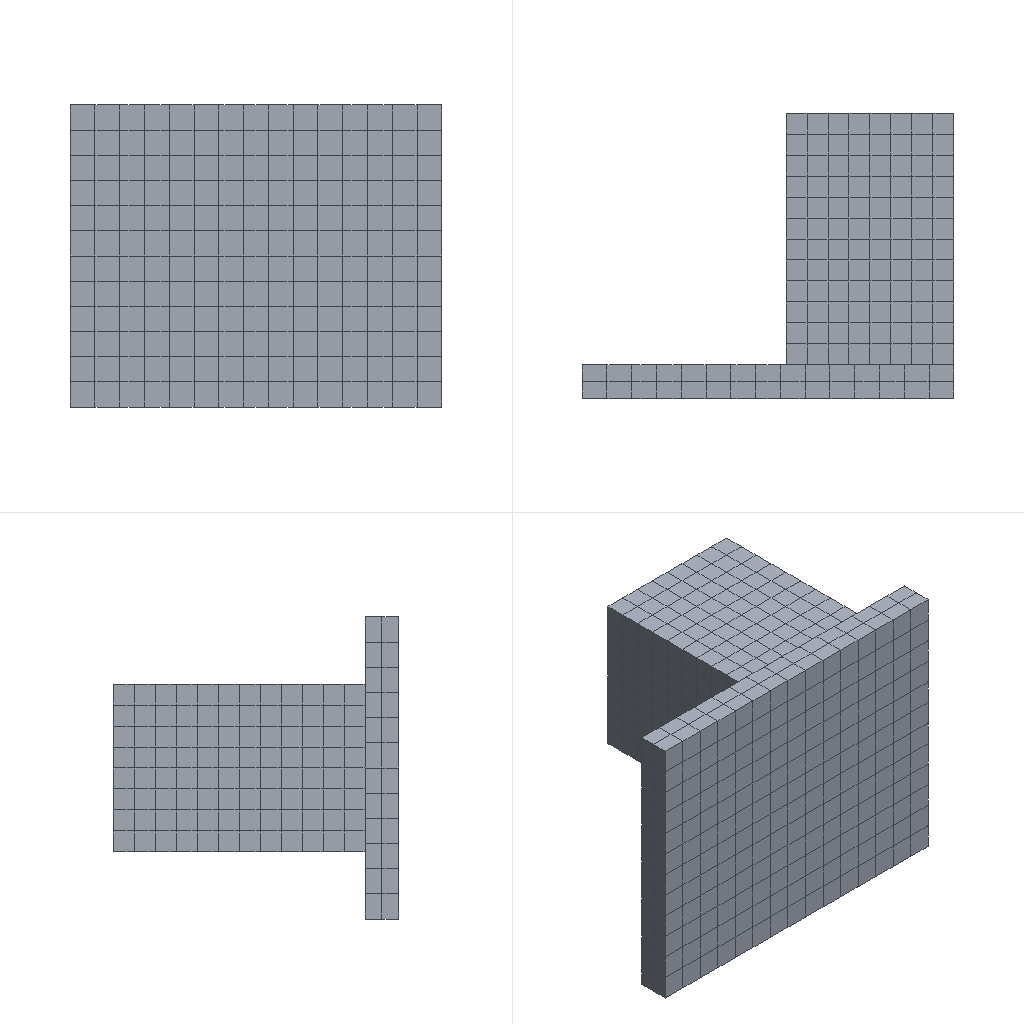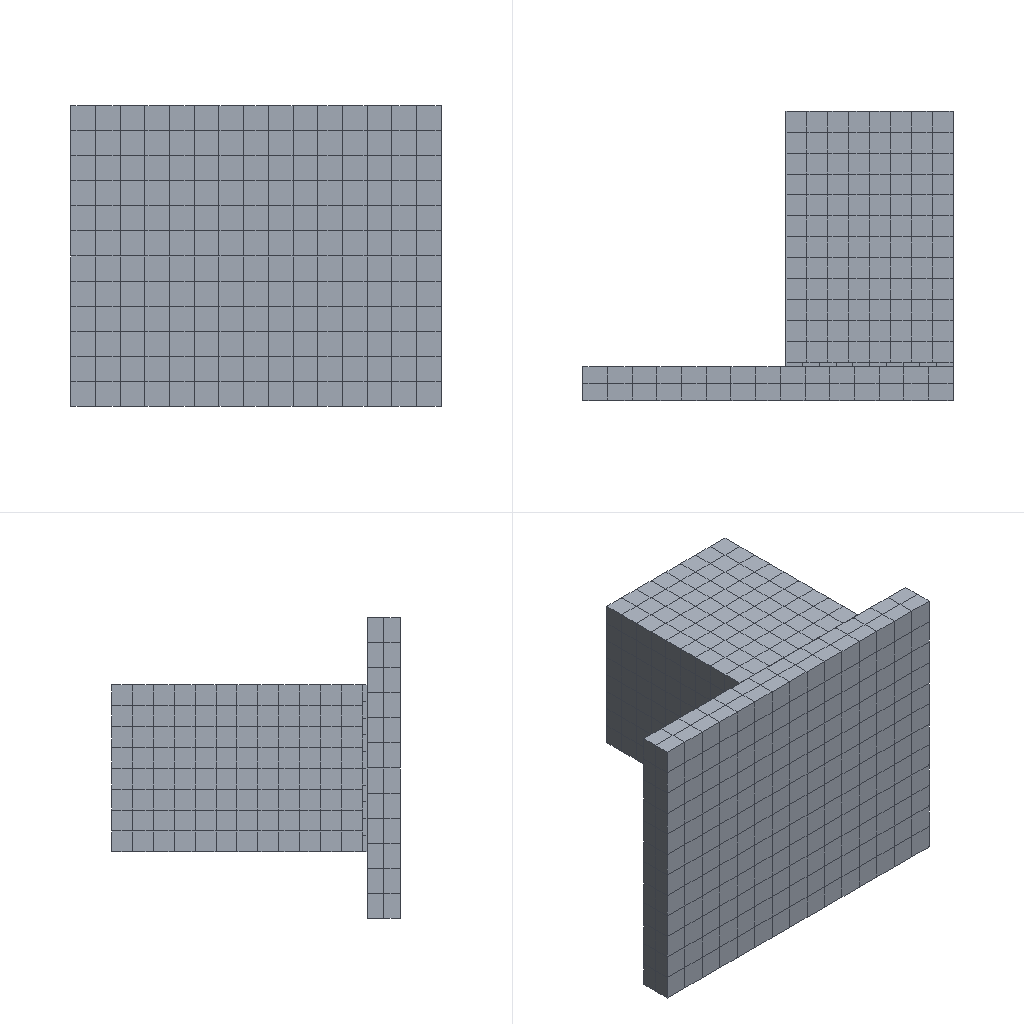Simulation study | ansys workbench
Set-up summary:
category,name,step,type,value,unit,region
solver,ansys_workbench
units,mm-N-s-tonne (MPa),,stated,"/units,MPA"
analysis,deck-1/LS1,,static
load_step,deck-1/LS1,deck-1/LS1,static,nsubst=5; time=1
analysis,deck-2/LS1,,static
load_step,deck-2/LS1,deck-2/LS1,static,nsubst=5; time=1
analysis,deck-3/LS1,,static
load_step,deck-3/LS1,deck-3/LS1,static,nsubst=5; time=1
mesh,deck-1.dat,,nodes,6098
mesh,deck-1.dat,,elements,1464
element_type,SOLID186,,,1128,,deck-1.dat
element_type,TARGE170,,,120,,deck-1.dat
element_type,CONTA174,,,120,,deck-1.dat
element_type,SURF154,,,96,,deck-1.dat
mesh,deck-2.dat,,nodes,6901
mesh,deck-2.dat,,elements,1974
element_type,SOLID186,,,1228,,deck-2.dat
element_type,TARGE170,,,320,,deck-2.dat
element_type,CONTA174,,,320,,deck-2.dat
element_type,SURF154,,,106,,deck-2.dat
mesh,deck-3.dat,,nodes,6901
mesh,deck-3.dat,,elements,1974
element_type,SOLID186,,,1228,,deck-3.dat
element_type,TARGE170,,,320,,deck-3.dat
element_type,CONTA174,,,320,,deck-3.dat
element_type,SURF154,,,106,,deck-3.dat
material,Structural Steel,,E,200000,tonne s^-2 mm^-1
material,Structural Steel,,nu,0.3
material,Structural Steel,,density,7.85e-09,tonne mm^-3
material,Structural Steel,,conductivity,60.5,tonne mm s^-3 C^-1
material,Structural Steel,,specific_heat,4.34e+08,mm^2 s^-2 C^-1
material,Structural Steel,,cte,1.2e-05,C^-1
material,Structural Steel,,permeability,10000
material,Structural Steel,,resistivity,0.00017,ohm mm
material,mat 3,,behaviors,"tb czm,CBDE"
material,Structural Steel,,E,200000,tonne s^-2 mm^-1
material,Structural Steel,,nu,0.3
material,Structural Steel,,density,7.85e-09,tonne mm^-3
material,Structural Steel,,conductivity,60.5,tonne mm s^-3 C^-1
material,Structural Steel,,specific_heat,4.34e+08,mm^2 s^-2 C^-1
material,Structural Steel,,cte,1.2e-05,C^-1
material,Structural Steel,,permeability,10000
material,Structural Steel,,resistivity,0.00017,ohm mm
material,mat 4,,behaviors,"tb czm,CBDE"
material,Structural Steel,,E,200000,tonne s^-2 mm^-1
material,Structural Steel,,nu,0.3
material,Structural Steel,,density,7.85e-09,tonne mm^-3
material,Structural Steel,,conductivity,60.5,tonne mm s^-3 C^-1
material,Structural Steel,,specific_heat,4.34e+08,mm^2 s^-2 C^-1
material,Structural Steel,,cte,1.2e-05,C^-1
material,Structural Steel,,permeability,10000
material,Structural Steel,,resistivity,0.00017,ohm mm
material,mat 4,,behaviors,"tb czm,CBDE"
load,Define Force Using Surface Effect Elements,deck-1/LS1,surface-effect pres face 1,133.333,,SURF154 #5
load,Define Force Using Surface Effect Elements,deck-1/LS1,surface-effect pres face 3,-2.31296e-14,,SURF154 #5
load,Define Force Using Surface Effect Elements,deck-2/LS1,surface-effect pres face 1,13.089,,SURF154 #8
load,Define Force Using Surface Effect Elements,deck-2/LS1,surface-effect pres face 3,-2.27058e-15,,SURF154 #8
load,Define Force Using Surface Effect Elements,deck-3/LS1,surface-effect pres face 1,13.089,,SURF154 #8
load,Define Force Using Surface Effect Elements,deck-3/LS1,surface-effect pres face 3,-2.27058e-15,,SURF154 #8
bc,Fixed Supports,deck-1/model,fixed,[dofs=ALL],,_FIXEDSU
bc,Fixed Supports,deck-2/model,fixed,[dofs=ALL],,_FIXEDSU
bc,Fixed Supports,deck-3/model,fixed,[dofs=ALL],,_FIXEDSU
contact,Contact Region,,bonded (always),element=CONTA174
contact,Contact Region,,bonded (always),element=CONTA174
contact,Contact Region 2,,bonded (always),element=CONTA174
contact,Contact Region,,bonded (always),element=CONTA174
contact,Contact Region 2,,bonded (always),element=CONTA174
named_set,_FIXEDSU,,node,595
named_set,_FIXEDSU,,node,595
named_set,_FIXEDSU,,node,595
Results summary:
result,analyses[0].index,,,1
result,analyses[0].system,,,SYS
result,analyses[0].deck,,,deck-1.dat
result,analyses[0].solve_status,,,completed
result,analyses[0].analysis_type,,,static
result,analyses[0].physics,,,mechanical
result,analyses[0].unit_system,,,"NMM: mm, ton, N, s, mV, mA, degC"
result,analyses[0].n_sets,,,6
result,analyses[0].load_steps[0].set,set=6,,6
result,analyses[0].load_steps[0].time_or_freq,set=6,,1
result,analyses[0].load_steps[0].max_displacement_magnitude,set=6,,0.1369
result,analyses[0].load_steps[0].max_von_mises_nodal,set=6,,2455.95
result,analyses[0].load_steps[0].reaction_force_sum_xyz[1],set=6,,-5000
result,analyses[0].load_steps[0].reaction_force_sum_xyz[2],set=6,,-4.89402e-12
result,analyses[0].load_steps[0].reaction_force_sum_xyz[3],set=6,,2.00683e-12
result,analyses[1].index,,,2
result,analyses[1].system,,,SYS-1
result,analyses[1].deck,,,deck-2.dat
result,analyses[1].solve_status,,,completed
result,analyses[1].analysis_type,,,static
result,analyses[1].physics,,,mechanical
result,analyses[1].unit_system,,,"NMM: mm, ton, N, s, mV, mA, degC"
result,analyses[1].n_sets,,,4
result,analyses[1].load_steps[0].set,set=4,,4
result,analyses[1].load_steps[0].time_or_freq,set=4,,1
result,analyses[1].load_steps[0].max_displacement_magnitude,set=4,,0.0863
result,analyses[1].load_steps[0].max_von_mises_nodal,set=4,,513.581
result,analyses[1].load_steps[0].reaction_force_sum_xyz[1],set=4,,-500
result,analyses[1].load_steps[0].reaction_force_sum_xyz[2],set=4,,-2.1036e-13
result,analyses[1].load_steps[0].reaction_force_sum_xyz[3],set=4,,5.10826e-13
result,analyses[2].index,,,3
result,analyses[2].system,,,SYS-2
result,analyses[2].deck,,,deck-3.dat
result,analyses[2].solve_status,,,completed
result,analyses[2].analysis_type,,,static
result,analyses[2].physics,,,mechanical
result,analyses[2].unit_system,,,"NMM: mm, ton, N, s, mV, mA, degC"
result,analyses[2].n_sets,,,4
result,analyses[2].load_steps[0].set,set=4,,4
result,analyses[2].load_steps[0].time_or_freq,set=4,,1
result,analyses[2].load_steps[0].max_displacement_magnitude,set=4,,0.0863
result,analyses[2].load_steps[0].max_von_mises_nodal,set=4,,513.581
result,analyses[2].load_steps[0].reaction_force_sum_xyz[1],set=4,,-500
result,analyses[2].load_steps[0].reaction_force_sum_xyz[2],set=4,,-2.1036e-13
result,analyses[2].load_steps[0].reaction_force_sum_xyz[3],set=4,,5.10826e-13